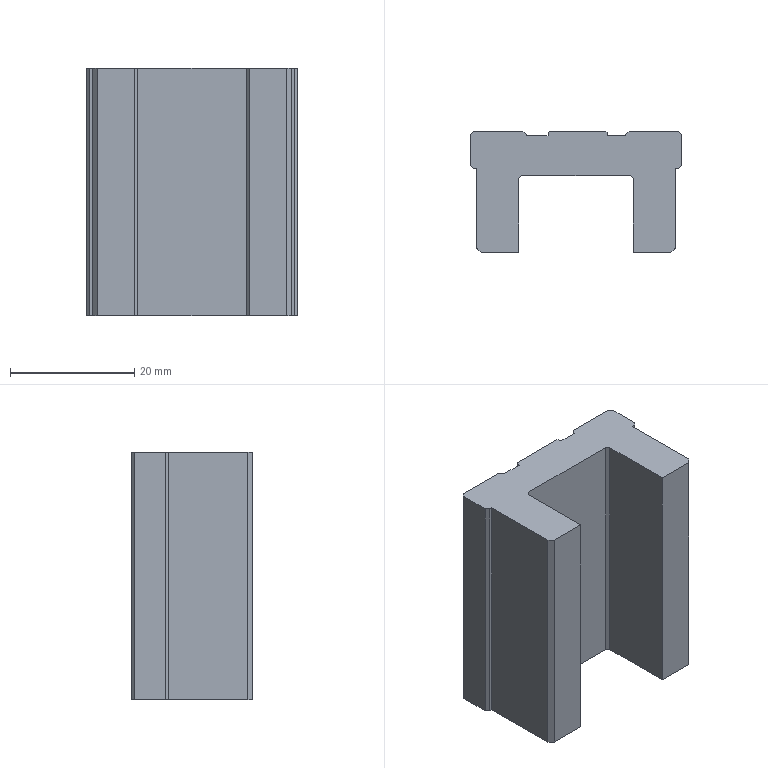Part | STEP file | 8 | 1 solid | 46 faces | box 34 x 19.5 x 39.8 mm | volume 15652 mm3 | plane 38 | cylinder 8 | commonest cylinder face diameters 4 x8
STEP:
#1=CARTESIAN_POINT('',(-13.,24.,-141.));
#2=VERTEX_POINT('',#1);
#3=CARTESIAN_POINT('',(-13.,24.,-145.));
#4=VERTEX_POINT('',#3);
#5=CARTESIAN_POINT('',(-13.,24.,-143.));
#6=DIRECTION('',(0.,-1.,0.));
#7=DIRECTION('',(0.,0.,-1.));
#8=AXIS2_PLACEMENT_3D('',#5,#6,#7);
#9=CIRCLE('',#8,2.);
#10=EDGE_CURVE('',#2,#4,#9,.T.);
#11=ORIENTED_EDGE('',*,*,#10,.F.);
#12=CARTESIAN_POINT('',(-13.,18.,-141.));
#13=VERTEX_POINT('',#12);
#14=CARTESIAN_POINT('',(-13.,24.,-141.));
#15=DIRECTION('',(0.,-1.,0.));
#16=VECTOR('',#15,1000.);
#17=LINE('',#14,#16);
#18=EDGE_CURVE('',#2,#13,#17,.T.);
#19=ORIENTED_EDGE('',*,*,#18,.T.);
#20=CARTESIAN_POINT('',(-13.,18.,-145.));
#21=VERTEX_POINT('',#20);
#22=CARTESIAN_POINT('',(-13.,18.,-143.));
#23=DIRECTION('',(0.,1.,0.));
#24=DIRECTION('',(0.,0.,-1.));
#25=AXIS2_PLACEMENT_3D('',#22,#23,#24);
#26=CIRCLE('',#25,2.);
#27=EDGE_CURVE('',#21,#13,#26,.T.);
#28=ORIENTED_EDGE('',*,*,#27,.F.);
#29=CARTESIAN_POINT('',(-13.,24.,-145.));
#30=DIRECTION('',(0.,-1.,0.));
#31=VECTOR('',#30,1000.);
#32=LINE('',#29,#31);
#33=EDGE_CURVE('',#4,#21,#32,.T.);
#34=ORIENTED_EDGE('',*,*,#33,.F.);
#35=EDGE_LOOP('',(#11,#19,#28,#34));
#36=FACE_OUTER_BOUND('',#35,.T.);
#37=CARTESIAN_POINT('',(-13.,24.,-143.));
#38=DIRECTION('',(0.,-1.,0.));
#39=DIRECTION('',(0.,0.,-1.));
#40=AXIS2_PLACEMENT_3D('',#37,#38,#39);
#41=CYLINDRICAL_SURFACE('',#40,2.);
#42=ADVANCED_FACE('',(#36),#41,.F.);
#43=CARTESIAN_POINT('',(-13.,24.,-115.));
#44=VERTEX_POINT('',#43);
#45=CARTESIAN_POINT('',(-13.,24.,-119.));
#46=VERTEX_POINT('',#45);
#47=CARTESIAN_POINT('',(-13.,24.,-117.));
#48=DIRECTION('',(0.,-1.,0.));
#49=DIRECTION('',(0.,0.,-1.));
#50=AXIS2_PLACEMENT_3D('',#47,#48,#49);
#51=CIRCLE('',#50,2.);
#52=EDGE_CURVE('',#44,#46,#51,.T.);
#53=ORIENTED_EDGE('',*,*,#52,.F.);
#54=CARTESIAN_POINT('',(-13.,18.,-115.));
#55=VERTEX_POINT('',#54);
#56=CARTESIAN_POINT('',(-13.,24.,-115.));
#57=DIRECTION('',(0.,-1.,0.));
#58=VECTOR('',#57,1000.);
#59=LINE('',#56,#58);
#60=EDGE_CURVE('',#44,#55,#59,.T.);
#61=ORIENTED_EDGE('',*,*,#60,.T.);
#62=CARTESIAN_POINT('',(-13.,18.,-119.));
#63=VERTEX_POINT('',#62);
#64=CARTESIAN_POINT('',(-13.,18.,-117.));
#65=DIRECTION('',(0.,1.,0.));
#66=DIRECTION('',(0.,0.,-1.));
#67=AXIS2_PLACEMENT_3D('',#64,#65,#66);
#68=CIRCLE('',#67,2.);
#69=EDGE_CURVE('',#63,#55,#68,.T.);
#70=ORIENTED_EDGE('',*,*,#69,.F.);
#71=CARTESIAN_POINT('',(-13.,24.,-119.));
#72=DIRECTION('',(0.,-1.,0.));
#73=VECTOR('',#72,1000.);
#74=LINE('',#71,#73);
#75=EDGE_CURVE('',#46,#63,#74,.T.);
#76=ORIENTED_EDGE('',*,*,#75,.F.);
#77=EDGE_LOOP('',(#53,#61,#70,#76));
#78=FACE_OUTER_BOUND('',#77,.T.);
#79=CARTESIAN_POINT('',(-13.,24.,-117.));
#80=DIRECTION('',(0.,-1.,0.));
#81=DIRECTION('',(0.,0.,-1.));
#82=AXIS2_PLACEMENT_3D('',#79,#80,#81);
#83=CYLINDRICAL_SURFACE('',#82,2.);
#84=ADVANCED_FACE('',(#78),#83,.F.);
#85=CARTESIAN_POINT('',(13.,24.,-115.));
#86=VERTEX_POINT('',#85);
#87=CARTESIAN_POINT('',(13.,24.,-119.));
#88=VERTEX_POINT('',#87);
#89=CARTESIAN_POINT('',(13.,24.,-117.));
#90=DIRECTION('',(0.,-1.,0.));
#91=DIRECTION('',(0.,0.,-1.));
#92=AXIS2_PLACEMENT_3D('',#89,#90,#91);
#93=CIRCLE('',#92,2.);
#94=EDGE_CURVE('',#86,#88,#93,.T.);
#95=ORIENTED_EDGE('',*,*,#94,.F.);
#96=CARTESIAN_POINT('',(13.,18.,-115.));
#97=VERTEX_POINT('',#96);
#98=CARTESIAN_POINT('',(13.,24.,-115.));
#99=DIRECTION('',(0.,-1.,0.));
#100=VECTOR('',#99,1000.);
#101=LINE('',#98,#100);
#102=EDGE_CURVE('',#86,#97,#101,.T.);
#103=ORIENTED_EDGE('',*,*,#102,.T.);
#104=CARTESIAN_POINT('',(13.,18.,-119.));
#105=VERTEX_POINT('',#104);
#106=CARTESIAN_POINT('',(13.,18.,-117.));
#107=DIRECTION('',(0.,1.,0.));
#108=DIRECTION('',(0.,0.,-1.));
#109=AXIS2_PLACEMENT_3D('',#106,#107,#108);
#110=CIRCLE('',#109,2.);
#111=EDGE_CURVE('',#105,#97,#110,.T.);
#112=ORIENTED_EDGE('',*,*,#111,.F.);
#113=CARTESIAN_POINT('',(13.,24.,-119.));
#114=DIRECTION('',(0.,-1.,0.));
#115=VECTOR('',#114,1000.);
#116=LINE('',#113,#115);
#117=EDGE_CURVE('',#88,#105,#116,.T.);
#118=ORIENTED_EDGE('',*,*,#117,.F.);
#119=EDGE_LOOP('',(#95,#103,#112,#118));
#120=FACE_OUTER_BOUND('',#119,.T.);
#121=CARTESIAN_POINT('',(13.,24.,-117.));
#122=DIRECTION('',(0.,-1.,0.));
#123=DIRECTION('',(0.,0.,-1.));
#124=AXIS2_PLACEMENT_3D('',#121,#122,#123);
#125=CYLINDRICAL_SURFACE('',#124,2.);
#126=ADVANCED_FACE('',(#120),#125,.F.);
#127=CARTESIAN_POINT('',(13.,24.,-141.));
#128=VERTEX_POINT('',#127);
#129=CARTESIAN_POINT('',(13.,24.,-145.));
#130=VERTEX_POINT('',#129);
#131=CARTESIAN_POINT('',(13.,24.,-143.));
#132=DIRECTION('',(0.,-1.,0.));
#133=DIRECTION('',(0.,0.,-1.));
#134=AXIS2_PLACEMENT_3D('',#131,#132,#133);
#135=CIRCLE('',#134,2.);
#136=EDGE_CURVE('',#128,#130,#135,.T.);
#137=ORIENTED_EDGE('',*,*,#136,.F.);
#138=CARTESIAN_POINT('',(13.,18.,-141.));
#139=VERTEX_POINT('',#138);
#140=CARTESIAN_POINT('',(13.,24.,-141.));
#141=DIRECTION('',(0.,-1.,0.));
#142=VECTOR('',#141,1000.);
#143=LINE('',#140,#142);
#144=EDGE_CURVE('',#128,#139,#143,.T.);
#145=ORIENTED_EDGE('',*,*,#144,.T.);
#146=CARTESIAN_POINT('',(13.,18.,-145.));
#147=VERTEX_POINT('',#146);
#148=CARTESIAN_POINT('',(13.,18.,-143.));
#149=DIRECTION('',(0.,1.,0.));
#150=DIRECTION('',(0.,0.,-1.));
#151=AXIS2_PLACEMENT_3D('',#148,#149,#150);
#152=CIRCLE('',#151,2.);
#153=EDGE_CURVE('',#147,#139,#152,.T.);
#154=ORIENTED_EDGE('',*,*,#153,.F.);
#155=CARTESIAN_POINT('',(13.,24.,-145.));
#156=DIRECTION('',(0.,-1.,0.));
#157=VECTOR('',#156,1000.);
#158=LINE('',#155,#157);
#159=EDGE_CURVE('',#130,#147,#158,.T.);
#160=ORIENTED_EDGE('',*,*,#159,.F.);
#161=EDGE_LOOP('',(#137,#145,#154,#160));
#162=FACE_OUTER_BOUND('',#161,.T.);
#163=CARTESIAN_POINT('',(13.,24.,-143.));
#164=DIRECTION('',(0.,-1.,0.));
#165=DIRECTION('',(0.,0.,-1.));
#166=AXIS2_PLACEMENT_3D('',#163,#164,#165);
#167=CYLINDRICAL_SURFACE('',#166,2.);
#168=ADVANCED_FACE('',(#162),#167,.F.);
#169=CARTESIAN_POINT('',(-8.75,16.9,-149.9));
#170=VERTEX_POINT('',#169);
#171=CARTESIAN_POINT('',(8.75,16.9,-149.9));
#172=VERTEX_POINT('',#171);
#173=CARTESIAN_POINT('',(0.,16.9,-149.9));
#174=DIRECTION('',(1.,0.,0.));
#175=VECTOR('',#174,1000.);
#176=LINE('',#173,#175);
#177=EDGE_CURVE('',#170,#172,#176,.T.);
#178=ORIENTED_EDGE('',*,*,#177,.T.);
#179=CARTESIAN_POINT('',(8.75,16.9,-110.1));
#180=VERTEX_POINT('',#179);
#181=CARTESIAN_POINT('',(8.75,16.9,-130.));
#182=DIRECTION('',(0.,0.,1.));
#183=VECTOR('',#182,1000.);
#184=LINE('',#181,#183);
#185=EDGE_CURVE('',#172,#180,#184,.T.);
#186=ORIENTED_EDGE('',*,*,#185,.T.);
#187=CARTESIAN_POINT('',(-8.75,16.9,-110.1));
#188=VERTEX_POINT('',#187);
#189=CARTESIAN_POINT('',(0.,16.9,-110.1));
#190=DIRECTION('',(-1.,0.,0.));
#191=VECTOR('',#190,1000.);
#192=LINE('',#189,#191);
#193=EDGE_CURVE('',#180,#188,#192,.T.);
#194=ORIENTED_EDGE('',*,*,#193,.T.);
#195=CARTESIAN_POINT('',(-8.75,16.9,-130.));
#196=DIRECTION('',(0.,0.,-1.));
#197=VECTOR('',#196,1000.);
#198=LINE('',#195,#197);
#199=EDGE_CURVE('',#188,#170,#198,.T.);
#200=ORIENTED_EDGE('',*,*,#199,.T.);
#201=EDGE_LOOP('',(#178,#186,#194,#200));
#202=FACE_OUTER_BOUND('',#201,.T.);
#203=CARTESIAN_POINT('',(0.,16.9,-130.));
#204=DIRECTION('',(0.,-1.,0.));
#205=DIRECTION('',(0.,0.,-1.));
#206=AXIS2_PLACEMENT_3D('',#203,#204,#205);
#207=PLANE('',#206);
#208=ADVANCED_FACE('',(#202),#207,.T.);
#209=CARTESIAN_POINT('',(9.25,16.4,-149.9));
#210=VERTEX_POINT('',#209);
#211=CARTESIAN_POINT('',(9.,16.65,-149.9));
#212=DIRECTION('',(0.7071,-0.7071,0.));
#213=VECTOR('',#212,1000.);
#214=LINE('',#211,#213);
#215=EDGE_CURVE('',#172,#210,#214,.T.);
#216=ORIENTED_EDGE('',*,*,#215,.T.);
#217=CARTESIAN_POINT('',(9.25,16.4,-110.1));
#218=VERTEX_POINT('',#217);
#219=CARTESIAN_POINT('',(9.25,16.4,-130.));
#220=DIRECTION('',(0.,0.,1.));
#221=VECTOR('',#220,1000.);
#222=LINE('',#219,#221);
#223=EDGE_CURVE('',#210,#218,#222,.T.);
#224=ORIENTED_EDGE('',*,*,#223,.T.);
#225=CARTESIAN_POINT('',(9.,16.65,-110.1));
#226=DIRECTION('',(-0.7071,0.7071,0.));
#227=VECTOR('',#226,1000.);
#228=LINE('',#225,#227);
#229=EDGE_CURVE('',#218,#180,#228,.T.);
#230=ORIENTED_EDGE('',*,*,#229,.T.);
#231=ORIENTED_EDGE('',*,*,#185,.F.);
#232=EDGE_LOOP('',(#216,#224,#230,#231));
#233=FACE_OUTER_BOUND('',#232,.T.);
#234=CARTESIAN_POINT('',(9.,16.65,-130.));
#235=DIRECTION('',(-0.7071,-0.7071,0.));
#236=DIRECTION('',(0.7071,-0.7071,0.));
#237=AXIS2_PLACEMENT_3D('',#234,#235,#236);
#238=PLANE('',#237);
#239=ADVANCED_FACE('',(#233),#238,.T.);
#240=ORIENTED_EDGE('',*,*,#177,.F.);
#241=CARTESIAN_POINT('',(-9.25,16.4,-149.9));
#242=VERTEX_POINT('',#241);
#243=CARTESIAN_POINT('',(-9.25,16.4,-149.9));
#244=DIRECTION('',(0.7071,0.7071,0.));
#245=VECTOR('',#244,1000.);
#246=LINE('',#243,#245);
#247=EDGE_CURVE('',#242,#170,#246,.T.);
#248=ORIENTED_EDGE('',*,*,#247,.F.);
#249=CARTESIAN_POINT('',(-9.25,4.5,-149.9));
#250=VERTEX_POINT('',#249);
#251=CARTESIAN_POINT('',(-9.25,15.226,-149.9));
#252=DIRECTION('',(0.,1.,0.));
#253=VECTOR('',#252,1000.);
#254=LINE('',#251,#253);
#255=EDGE_CURVE('',#250,#242,#254,.T.);
#256=ORIENTED_EDGE('',*,*,#255,.F.);
#257=CARTESIAN_POINT('',(-15.25,4.5,-149.9));
#258=VERTEX_POINT('',#257);
#259=CARTESIAN_POINT('',(0.002327,4.5,-149.9));
#260=DIRECTION('',(1.,0.,0.));
#261=VECTOR('',#260,1000.);
#262=LINE('',#259,#261);
#263=EDGE_CURVE('',#258,#250,#262,.T.);
#264=ORIENTED_EDGE('',*,*,#263,.F.);
#265=CARTESIAN_POINT('',(-16.,5.25,-149.9));
#266=VERTEX_POINT('',#265);
#267=CARTESIAN_POINT('',(-15.625,4.875,-149.9));
#268=DIRECTION('',(0.7071,-0.7071,0.));
#269=VECTOR('',#268,1000.);
#270=LINE('',#267,#269);
#271=EDGE_CURVE('',#266,#258,#270,.T.);
#272=ORIENTED_EDGE('',*,*,#271,.F.);
#273=CARTESIAN_POINT('',(-16.,18.,-149.9));
#274=VERTEX_POINT('',#273);
#275=CARTESIAN_POINT('',(-16.,15.226,-149.9));
#276=DIRECTION('',(0.,-1.,0.));
#277=VECTOR('',#276,1000.);
#278=LINE('',#275,#277);
#279=EDGE_CURVE('',#274,#266,#278,.T.);
#280=ORIENTED_EDGE('',*,*,#279,.F.);
#281=CARTESIAN_POINT('',(-16.5,18.,-149.9));
#282=VERTEX_POINT('',#281);
#283=CARTESIAN_POINT('',(-16.25,18.,-149.9));
#284=DIRECTION('',(1.,0.,0.));
#285=VECTOR('',#284,1000.);
#286=LINE('',#283,#285);
#287=EDGE_CURVE('',#282,#274,#286,.T.);
#288=ORIENTED_EDGE('',*,*,#287,.F.);
#289=CARTESIAN_POINT('',(-17.,18.5,-149.9));
#290=VERTEX_POINT('',#289);
#291=CARTESIAN_POINT('',(-16.75,18.25,-149.9));
#292=DIRECTION('',(0.7071,-0.7071,0.));
#293=VECTOR('',#292,1000.);
#294=LINE('',#291,#293);
#295=EDGE_CURVE('',#290,#282,#294,.T.);
#296=ORIENTED_EDGE('',*,*,#295,.F.);
#297=CARTESIAN_POINT('',(-17.,23.5,-149.9));
#298=VERTEX_POINT('',#297);
#299=CARTESIAN_POINT('',(-17.,15.226,-149.9));
#300=DIRECTION('',(0.,-1.,0.));
#301=VECTOR('',#300,1000.);
#302=LINE('',#299,#301);
#303=EDGE_CURVE('',#298,#290,#302,.T.);
#304=ORIENTED_EDGE('',*,*,#303,.F.);
#305=CARTESIAN_POINT('',(-16.5,24.,-149.9));
#306=VERTEX_POINT('',#305);
#307=CARTESIAN_POINT('',(-16.75,23.75,-149.9));
#308=DIRECTION('',(-0.7071,-0.7071,0.));
#309=VECTOR('',#308,1000.);
#310=LINE('',#307,#309);
#311=EDGE_CURVE('',#306,#298,#310,.T.);
#312=ORIENTED_EDGE('',*,*,#311,.F.);
#313=CARTESIAN_POINT('',(-8.707,24.,-149.9));
#314=VERTEX_POINT('',#313);
#315=CARTESIAN_POINT('',(0.002327,24.,-149.9));
#316=DIRECTION('',(-1.,0.,0.));
#317=VECTOR('',#316,1000.);
#318=LINE('',#315,#317);
#319=EDGE_CURVE('',#314,#306,#318,.T.);
#320=ORIENTED_EDGE('',*,*,#319,.F.);
#321=CARTESIAN_POINT('',(-8.,23.5,-149.9));
#322=VERTEX_POINT('',#321);
#323=CARTESIAN_POINT('',(-8.354,23.75,-149.9));
#324=DIRECTION('',(-0.8165,0.5774,0.));
#325=VECTOR('',#324,1000.);
#326=LINE('',#323,#325);
#327=EDGE_CURVE('',#322,#314,#326,.T.);
#328=ORIENTED_EDGE('',*,*,#327,.F.);
#329=CARTESIAN_POINT('',(-8.,23.3,-149.9));
#330=VERTEX_POINT('',#329);
#331=CARTESIAN_POINT('',(-8.,23.4,-149.9));
#332=DIRECTION('',(0.,1.,0.));
#333=VECTOR('',#332,1000.);
#334=LINE('',#331,#333);
#335=EDGE_CURVE('',#330,#322,#334,.T.);
#336=ORIENTED_EDGE('',*,*,#335,.F.);
#337=CARTESIAN_POINT('',(-4.5,23.3,-149.9));
#338=VERTEX_POINT('',#337);
#339=CARTESIAN_POINT('',(0.002327,23.3,-149.9));
#340=DIRECTION('',(-1.,0.,0.));
#341=VECTOR('',#340,1000.);
#342=LINE('',#339,#341);
#343=EDGE_CURVE('',#338,#330,#342,.T.);
#344=ORIENTED_EDGE('',*,*,#343,.F.);
#345=CARTESIAN_POINT('',(-4.5,23.8,-149.9));
#346=VERTEX_POINT('',#345);
#347=CARTESIAN_POINT('',(-4.5,23.55,-149.9));
#348=DIRECTION('',(0.,-1.,0.));
#349=VECTOR('',#348,1000.);
#350=LINE('',#347,#349);
#351=EDGE_CURVE('',#346,#338,#350,.T.);
#352=ORIENTED_EDGE('',*,*,#351,.F.);
#353=CARTESIAN_POINT('',(-4.3,24.,-149.9));
#354=VERTEX_POINT('',#353);
#355=CARTESIAN_POINT('',(-4.4,23.9,-149.9));
#356=DIRECTION('',(-0.7071,-0.7071,0.));
#357=VECTOR('',#356,1000.);
#358=LINE('',#355,#357);
#359=EDGE_CURVE('',#354,#346,#358,.T.);
#360=ORIENTED_EDGE('',*,*,#359,.F.);
#361=CARTESIAN_POINT('',(4.8,24.,-149.9));
#362=VERTEX_POINT('',#361);
#363=CARTESIAN_POINT('',(0.002327,24.,-149.9));
#364=DIRECTION('',(-1.,0.,0.));
#365=VECTOR('',#364,1000.);
#366=LINE('',#363,#365);
#367=EDGE_CURVE('',#362,#354,#366,.T.);
#368=ORIENTED_EDGE('',*,*,#367,.F.);
#369=CARTESIAN_POINT('',(5.,23.8,-149.9));
#370=VERTEX_POINT('',#369);
#371=CARTESIAN_POINT('',(4.9,23.9,-149.9));
#372=DIRECTION('',(-0.7071,0.7071,0.));
#373=VECTOR('',#372,1000.);
#374=LINE('',#371,#373);
#375=EDGE_CURVE('',#370,#362,#374,.T.);
#376=ORIENTED_EDGE('',*,*,#375,.F.);
#377=CARTESIAN_POINT('',(5.,23.3,-149.9));
#378=VERTEX_POINT('',#377);
#379=CARTESIAN_POINT('',(5.,23.55,-149.9));
#380=DIRECTION('',(0.,1.,0.));
#381=VECTOR('',#380,1000.);
#382=LINE('',#379,#381);
#383=EDGE_CURVE('',#378,#370,#382,.T.);
#384=ORIENTED_EDGE('',*,*,#383,.F.);
#385=CARTESIAN_POINT('',(8.,23.3,-149.9));
#386=VERTEX_POINT('',#385);
#387=CARTESIAN_POINT('',(0.002327,23.3,-149.9));
#388=DIRECTION('',(-1.,0.,0.));
#389=VECTOR('',#388,1000.);
#390=LINE('',#387,#389);
#391=EDGE_CURVE('',#386,#378,#390,.T.);
#392=ORIENTED_EDGE('',*,*,#391,.F.);
#393=CARTESIAN_POINT('',(8.,23.5,-149.9));
#394=VERTEX_POINT('',#393);
#395=CARTESIAN_POINT('',(8.,23.4,-149.9));
#396=DIRECTION('',(0.,-1.,0.));
#397=VECTOR('',#396,1000.);
#398=LINE('',#395,#397);
#399=EDGE_CURVE('',#394,#386,#398,.T.);
#400=ORIENTED_EDGE('',*,*,#399,.F.);
#401=CARTESIAN_POINT('',(8.707,24.,-149.9));
#402=VERTEX_POINT('',#401);
#403=CARTESIAN_POINT('',(8.354,23.75,-149.9));
#404=DIRECTION('',(-0.8165,-0.5774,0.));
#405=VECTOR('',#404,1000.);
#406=LINE('',#403,#405);
#407=EDGE_CURVE('',#402,#394,#406,.T.);
#408=ORIENTED_EDGE('',*,*,#407,.F.);
#409=CARTESIAN_POINT('',(16.5,24.,-149.9));
#410=VERTEX_POINT('',#409);
#411=CARTESIAN_POINT('',(0.002327,24.,-149.9));
#412=DIRECTION('',(-1.,0.,0.));
#413=VECTOR('',#412,1000.);
#414=LINE('',#411,#413);
#415=EDGE_CURVE('',#410,#402,#414,.T.);
#416=ORIENTED_EDGE('',*,*,#415,.F.);
#417=CARTESIAN_POINT('',(17.,23.5,-149.9));
#418=VERTEX_POINT('',#417);
#419=CARTESIAN_POINT('',(16.75,23.75,-149.9));
#420=DIRECTION('',(-0.7071,0.7071,0.));
#421=VECTOR('',#420,1000.);
#422=LINE('',#419,#421);
#423=EDGE_CURVE('',#418,#410,#422,.T.);
#424=ORIENTED_EDGE('',*,*,#423,.F.);
#425=CARTESIAN_POINT('',(17.,18.5,-149.9));
#426=VERTEX_POINT('',#425);
#427=CARTESIAN_POINT('',(17.,15.226,-149.9));
#428=DIRECTION('',(0.,1.,0.));
#429=VECTOR('',#428,1000.);
#430=LINE('',#427,#429);
#431=EDGE_CURVE('',#426,#418,#430,.T.);
#432=ORIENTED_EDGE('',*,*,#431,.F.);
#433=CARTESIAN_POINT('',(16.5,18.,-149.9));
#434=VERTEX_POINT('',#433);
#435=CARTESIAN_POINT('',(16.75,18.25,-149.9));
#436=DIRECTION('',(0.7071,0.7071,0.));
#437=VECTOR('',#436,1000.);
#438=LINE('',#435,#437);
#439=EDGE_CURVE('',#434,#426,#438,.T.);
#440=ORIENTED_EDGE('',*,*,#439,.F.);
#441=CARTESIAN_POINT('',(16.,18.,-149.9));
#442=VERTEX_POINT('',#441);
#443=CARTESIAN_POINT('',(16.25,18.,-149.9));
#444=DIRECTION('',(1.,0.,0.));
#445=VECTOR('',#444,1000.);
#446=LINE('',#443,#445);
#447=EDGE_CURVE('',#442,#434,#446,.T.);
#448=ORIENTED_EDGE('',*,*,#447,.F.);
#449=CARTESIAN_POINT('',(16.,5.25,-149.9));
#450=VERTEX_POINT('',#449);
#451=CARTESIAN_POINT('',(16.,15.226,-149.9));
#452=DIRECTION('',(0.,1.,0.));
#453=VECTOR('',#452,1000.);
#454=LINE('',#451,#453);
#455=EDGE_CURVE('',#450,#442,#454,.T.);
#456=ORIENTED_EDGE('',*,*,#455,.F.);
#457=CARTESIAN_POINT('',(15.25,4.5,-149.9));
#458=VERTEX_POINT('',#457);
#459=CARTESIAN_POINT('',(15.625,4.875,-149.9));
#460=DIRECTION('',(0.7071,0.7071,0.));
#461=VECTOR('',#460,1000.);
#462=LINE('',#459,#461);
#463=EDGE_CURVE('',#458,#450,#462,.T.);
#464=ORIENTED_EDGE('',*,*,#463,.F.);
#465=CARTESIAN_POINT('',(9.25,4.5,-149.9));
#466=VERTEX_POINT('',#465);
#467=CARTESIAN_POINT('',(0.002327,4.5,-149.9));
#468=DIRECTION('',(1.,0.,0.));
#469=VECTOR('',#468,1000.);
#470=LINE('',#467,#469);
#471=EDGE_CURVE('',#466,#458,#470,.T.);
#472=ORIENTED_EDGE('',*,*,#471,.F.);
#473=CARTESIAN_POINT('',(9.25,15.226,-149.9));
#474=DIRECTION('',(0.,-1.,0.));
#475=VECTOR('',#474,1000.);
#476=LINE('',#473,#475);
#477=EDGE_CURVE('',#210,#466,#476,.T.);
#478=ORIENTED_EDGE('',*,*,#477,.F.);
#479=ORIENTED_EDGE('',*,*,#215,.F.);
#480=EDGE_LOOP('',(#240,#248,#256,#264,#272,#280,#288,#296,#304,#312,#320,#328,#336,#344,#352,#360,#368,#376,#384,#392,#400,#408,#416,#424,#432,#440,#448,#456,#464,#472,#478,#479));
#481=FACE_OUTER_BOUND('',#480,.T.);
#482=CARTESIAN_POINT('',(0.002327,15.226,-149.9));
#483=DIRECTION('',(0.,0.,1.));
#484=DIRECTION('',(0.,-1.,0.));
#485=AXIS2_PLACEMENT_3D('',#482,#483,#484);
#486=PLANE('',#485);
#487=ADVANCED_FACE('',(#481),#486,.F.);
#488=ORIENTED_EDGE('',*,*,#247,.T.);
#489=ORIENTED_EDGE('',*,*,#199,.F.);
#490=CARTESIAN_POINT('',(-9.25,16.4,-110.1));
#491=VERTEX_POINT('',#490);
#492=CARTESIAN_POINT('',(-9.,16.65,-110.1));
#493=DIRECTION('',(-0.7071,-0.7071,0.));
#494=VECTOR('',#493,1000.);
#495=LINE('',#492,#494);
#496=EDGE_CURVE('',#188,#491,#495,.T.);
#497=ORIENTED_EDGE('',*,*,#496,.T.);
#498=CARTESIAN_POINT('',(-9.25,16.4,-130.));
#499=DIRECTION('',(0.,0.,-1.));
#500=VECTOR('',#499,1000.);
#501=LINE('',#498,#500);
#502=EDGE_CURVE('',#491,#242,#501,.T.);
#503=ORIENTED_EDGE('',*,*,#502,.T.);
#504=EDGE_LOOP('',(#488,#489,#497,#503));
#505=FACE_OUTER_BOUND('',#504,.T.);
#506=CARTESIAN_POINT('',(-9.,16.65,-130.));
#507=DIRECTION('',(0.7071,-0.7071,0.));
#508=DIRECTION('',(0.7071,0.7071,0.));
#509=AXIS2_PLACEMENT_3D('',#506,#507,#508);
#510=PLANE('',#509);
#511=ADVANCED_FACE('',(#505),#510,.T.);
#512=CARTESIAN_POINT('',(-15.25,4.5,-110.1));
#513=VERTEX_POINT('',#512);
#514=CARTESIAN_POINT('',(-9.25,4.5,-110.1));
#515=VERTEX_POINT('',#514);
#516=CARTESIAN_POINT('',(0.002327,4.5,-110.1));
#517=DIRECTION('',(1.,0.,0.));
#518=VECTOR('',#517,1000.);
#519=LINE('',#516,#518);
#520=EDGE_CURVE('',#513,#515,#519,.T.);
#521=ORIENTED_EDGE('',*,*,#520,.T.);
#522=CARTESIAN_POINT('',(-9.25,15.226,-110.1));
#523=DIRECTION('',(0.,1.,0.));
#524=VECTOR('',#523,1000.);
#525=LINE('',#522,#524);
#526=EDGE_CURVE('',#515,#491,#525,.T.);
#527=ORIENTED_EDGE('',*,*,#526,.T.);
#528=ORIENTED_EDGE('',*,*,#496,.F.);
#529=ORIENTED_EDGE('',*,*,#193,.F.);
#530=ORIENTED_EDGE('',*,*,#229,.F.);
#531=CARTESIAN_POINT('',(9.25,4.5,-110.1));
#532=VERTEX_POINT('',#531);
#533=CARTESIAN_POINT('',(9.25,15.226,-110.1));
#534=DIRECTION('',(0.,-1.,0.));
#535=VECTOR('',#534,1000.);
#536=LINE('',#533,#535);
#537=EDGE_CURVE('',#218,#532,#536,.T.);
#538=ORIENTED_EDGE('',*,*,#537,.T.);
#539=CARTESIAN_POINT('',(15.25,4.5,-110.1));
#540=VERTEX_POINT('',#539);
#541=CARTESIAN_POINT('',(0.002327,4.5,-110.1));
#542=DIRECTION('',(1.,0.,0.));
#543=VECTOR('',#542,1000.);
#544=LINE('',#541,#543);
#545=EDGE_CURVE('',#532,#540,#544,.T.);
#546=ORIENTED_EDGE('',*,*,#545,.T.);
#547=CARTESIAN_POINT('',(16.,5.25,-110.1));
#548=VERTEX_POINT('',#547);
#549=CARTESIAN_POINT('',(15.625,4.875,-110.1));
#550=DIRECTION('',(-0.7071,-0.7071,0.));
#551=VECTOR('',#550,1000.);
#552=LINE('',#549,#551);
#553=EDGE_CURVE('',#548,#540,#552,.T.);
#554=ORIENTED_EDGE('',*,*,#553,.F.);
#555=CARTESIAN_POINT('',(16.,18.,-110.1));
#556=VERTEX_POINT('',#555);
#557=CARTESIAN_POINT('',(16.,15.226,-110.1));
#558=DIRECTION('',(0.,1.,0.));
#559=VECTOR('',#558,1000.);
#560=LINE('',#557,#559);
#561=EDGE_CURVE('',#548,#556,#560,.T.);
#562=ORIENTED_EDGE('',*,*,#561,.T.);
#563=CARTESIAN_POINT('',(16.5,18.,-110.1));
#564=VERTEX_POINT('',#563);
#565=CARTESIAN_POINT('',(16.25,18.,-110.1));
#566=DIRECTION('',(-1.,0.,0.));
#567=VECTOR('',#566,1000.);
#568=LINE('',#565,#567);
#569=EDGE_CURVE('',#564,#556,#568,.T.);
#570=ORIENTED_EDGE('',*,*,#569,.F.);
#571=CARTESIAN_POINT('',(17.,18.5,-110.1));
#572=VERTEX_POINT('',#571);
#573=CARTESIAN_POINT('',(16.75,18.25,-110.1));
#574=DIRECTION('',(-0.7071,-0.7071,0.));
#575=VECTOR('',#574,1000.);
#576=LINE('',#573,#575);
#577=EDGE_CURVE('',#572,#564,#576,.T.);
#578=ORIENTED_EDGE('',*,*,#577,.F.);
#579=CARTESIAN_POINT('',(17.,23.5,-110.1));
#580=VERTEX_POINT('',#579);
#581=CARTESIAN_POINT('',(17.,15.226,-110.1));
#582=DIRECTION('',(0.,1.,0.));
#583=VECTOR('',#582,1000.);
#584=LINE('',#581,#583);
#585=EDGE_CURVE('',#572,#580,#584,.T.);
#586=ORIENTED_EDGE('',*,*,#585,.T.);
#587=CARTESIAN_POINT('',(16.5,24.,-110.1));
#588=VERTEX_POINT('',#587);
#589=CARTESIAN_POINT('',(16.75,23.75,-110.1));
#590=DIRECTION('',(0.7071,-0.7071,0.));
#591=VECTOR('',#590,1000.);
#592=LINE('',#589,#591);
#593=EDGE_CURVE('',#588,#580,#592,.T.);
#594=ORIENTED_EDGE('',*,*,#593,.F.);
#595=CARTESIAN_POINT('',(8.707,24.,-110.1));
#596=VERTEX_POINT('',#595);
#597=CARTESIAN_POINT('',(0.002327,24.,-110.1));
#598=DIRECTION('',(-1.,0.,0.));
#599=VECTOR('',#598,1000.);
#600=LINE('',#597,#599);
#601=EDGE_CURVE('',#588,#596,#600,.T.);
#602=ORIENTED_EDGE('',*,*,#601,.T.);
#603=CARTESIAN_POINT('',(8.,23.5,-110.1));
#604=VERTEX_POINT('',#603);
#605=CARTESIAN_POINT('',(8.354,23.75,-110.1));
#606=DIRECTION('',(0.8165,0.5774,0.));
#607=VECTOR('',#606,1000.);
#608=LINE('',#605,#607);
#609=EDGE_CURVE('',#604,#596,#608,.T.);
#610=ORIENTED_EDGE('',*,*,#609,.F.);
#611=CARTESIAN_POINT('',(8.,23.3,-110.1));
#612=VERTEX_POINT('',#611);
#613=CARTESIAN_POINT('',(8.,23.4,-110.1));
#614=DIRECTION('',(0.,1.,0.));
#615=VECTOR('',#614,1000.);
#616=LINE('',#613,#615);
#617=EDGE_CURVE('',#612,#604,#616,.T.);
#618=ORIENTED_EDGE('',*,*,#617,.F.);
#619=CARTESIAN_POINT('',(5.,23.3,-110.1));
#620=VERTEX_POINT('',#619);
#621=CARTESIAN_POINT('',(0.002327,23.3,-110.1));
#622=DIRECTION('',(-1.,0.,0.));
#623=VECTOR('',#622,1000.);
#624=LINE('',#621,#623);
#625=EDGE_CURVE('',#612,#620,#624,.T.);
#626=ORIENTED_EDGE('',*,*,#625,.T.);
#627=CARTESIAN_POINT('',(5.,23.8,-110.1));
#628=VERTEX_POINT('',#627);
#629=CARTESIAN_POINT('',(5.,23.55,-110.1));
#630=DIRECTION('',(0.,-1.,0.));
#631=VECTOR('',#630,1000.);
#632=LINE('',#629,#631);
#633=EDGE_CURVE('',#628,#620,#632,.T.);
#634=ORIENTED_EDGE('',*,*,#633,.F.);
#635=CARTESIAN_POINT('',(4.8,24.,-110.1));
#636=VERTEX_POINT('',#635);
#637=CARTESIAN_POINT('',(4.9,23.9,-110.1));
#638=DIRECTION('',(0.7071,-0.7071,0.));
#639=VECTOR('',#638,1000.);
#640=LINE('',#637,#639);
#641=EDGE_CURVE('',#636,#628,#640,.T.);
#642=ORIENTED_EDGE('',*,*,#641,.F.);
#643=CARTESIAN_POINT('',(-4.3,24.,-110.1));
#644=VERTEX_POINT('',#643);
#645=CARTESIAN_POINT('',(0.002327,24.,-110.1));
#646=DIRECTION('',(-1.,0.,0.));
#647=VECTOR('',#646,1000.);
#648=LINE('',#645,#647);
#649=EDGE_CURVE('',#636,#644,#648,.T.);
#650=ORIENTED_EDGE('',*,*,#649,.T.);
#651=CARTESIAN_POINT('',(-4.5,23.8,-110.1));
#652=VERTEX_POINT('',#651);
#653=CARTESIAN_POINT('',(-4.4,23.9,-110.1));
#654=DIRECTION('',(0.7071,0.7071,0.));
#655=VECTOR('',#654,1000.);
#656=LINE('',#653,#655);
#657=EDGE_CURVE('',#652,#644,#656,.T.);
#658=ORIENTED_EDGE('',*,*,#657,.F.);
#659=CARTESIAN_POINT('',(-4.5,23.3,-110.1));
#660=VERTEX_POINT('',#659);
#661=CARTESIAN_POINT('',(-4.5,23.55,-110.1));
#662=DIRECTION('',(0.,1.,0.));
#663=VECTOR('',#662,1000.);
#664=LINE('',#661,#663);
#665=EDGE_CURVE('',#660,#652,#664,.T.);
#666=ORIENTED_EDGE('',*,*,#665,.F.);
#667=CARTESIAN_POINT('',(-8.,23.3,-110.1));
#668=VERTEX_POINT('',#667);
#669=CARTESIAN_POINT('',(0.002327,23.3,-110.1));
#670=DIRECTION('',(-1.,0.,0.));
#671=VECTOR('',#670,1000.);
#672=LINE('',#669,#671);
#673=EDGE_CURVE('',#660,#668,#672,.T.);
#674=ORIENTED_EDGE('',*,*,#673,.T.);
#675=CARTESIAN_POINT('',(-8.,23.5,-110.1));
#676=VERTEX_POINT('',#675);
#677=CARTESIAN_POINT('',(-8.,23.4,-110.1));
#678=DIRECTION('',(0.,-1.,0.));
#679=VECTOR('',#678,1000.);
#680=LINE('',#677,#679);
#681=EDGE_CURVE('',#676,#668,#680,.T.);
#682=ORIENTED_EDGE('',*,*,#681,.F.);
#683=CARTESIAN_POINT('',(-8.707,24.,-110.1));
#684=VERTEX_POINT('',#683);
#685=CARTESIAN_POINT('',(-8.354,23.75,-110.1));
#686=DIRECTION('',(0.8165,-0.5774,0.));
#687=VECTOR('',#686,1000.);
#688=LINE('',#685,#687);
#689=EDGE_CURVE('',#684,#676,#688,.T.);
#690=ORIENTED_EDGE('',*,*,#689,.F.);
#691=CARTESIAN_POINT('',(-16.5,24.,-110.1));
#692=VERTEX_POINT('',#691);
#693=CARTESIAN_POINT('',(0.002327,24.,-110.1));
#694=DIRECTION('',(-1.,0.,0.));
#695=VECTOR('',#694,1000.);
#696=LINE('',#693,#695);
#697=EDGE_CURVE('',#684,#692,#696,.T.);
#698=ORIENTED_EDGE('',*,*,#697,.T.);
#699=CARTESIAN_POINT('',(-17.,23.5,-110.1));
#700=VERTEX_POINT('',#699);
#701=CARTESIAN_POINT('',(-16.75,23.75,-110.1));
#702=DIRECTION('',(0.7071,0.7071,0.));
#703=VECTOR('',#702,1000.);
#704=LINE('',#701,#703);
#705=EDGE_CURVE('',#700,#692,#704,.T.);
#706=ORIENTED_EDGE('',*,*,#705,.F.);
#707=CARTESIAN_POINT('',(-17.,18.5,-110.1));
#708=VERTEX_POINT('',#707);
#709=CARTESIAN_POINT('',(-17.,15.226,-110.1));
#710=DIRECTION('',(0.,-1.,0.));
#711=VECTOR('',#710,1000.);
#712=LINE('',#709,#711);
#713=EDGE_CURVE('',#700,#708,#712,.T.);
#714=ORIENTED_EDGE('',*,*,#713,.T.);
#715=CARTESIAN_POINT('',(-16.5,18.,-110.1));
#716=VERTEX_POINT('',#715);
#717=CARTESIAN_POINT('',(-16.75,18.25,-110.1));
#718=DIRECTION('',(-0.7071,0.7071,0.));
#719=VECTOR('',#718,1000.);
#720=LINE('',#717,#719);
#721=EDGE_CURVE('',#716,#708,#720,.T.);
#722=ORIENTED_EDGE('',*,*,#721,.F.);
#723=CARTESIAN_POINT('',(-16.,18.,-110.1));
#724=VERTEX_POINT('',#723);
#725=CARTESIAN_POINT('',(-16.25,18.,-110.1));
#726=DIRECTION('',(-1.,0.,0.));
#727=VECTOR('',#726,1000.);
#728=LINE('',#725,#727);
#729=EDGE_CURVE('',#724,#716,#728,.T.);
#730=ORIENTED_EDGE('',*,*,#729,.F.);
#731=CARTESIAN_POINT('',(-16.,5.25,-110.1));
#732=VERTEX_POINT('',#731);
#733=CARTESIAN_POINT('',(-16.,15.226,-110.1));
#734=DIRECTION('',(0.,-1.,0.));
#735=VECTOR('',#734,1000.);
#736=LINE('',#733,#735);
#737=EDGE_CURVE('',#724,#732,#736,.T.);
#738=ORIENTED_EDGE('',*,*,#737,.T.);
#739=CARTESIAN_POINT('',(-15.625,4.875,-110.1));
#740=DIRECTION('',(-0.7071,0.7071,0.));
#741=VECTOR('',#740,1000.);
#742=LINE('',#739,#741);
#743=EDGE_CURVE('',#513,#732,#742,.T.);
#744=ORIENTED_EDGE('',*,*,#743,.F.);
#745=EDGE_LOOP('',(#521,#527,#528,#529,#530,#538,#546,#554,#562,#570,#578,#586,#594,#602,#610,#618,#626,#634,#642,#650,#658,#666,#674,#682,#690,#698,#706,#714,#722,#730,#738,#744));
#746=FACE_OUTER_BOUND('',#745,.T.);
#747=CARTESIAN_POINT('',(0.002327,15.226,-110.1));
#748=DIRECTION('',(0.,0.,1.));
#749=DIRECTION('',(0.,-1.,0.));
#750=AXIS2_PLACEMENT_3D('',#747,#748,#749);
#751=PLANE('',#750);
#752=ADVANCED_FACE('',(#746),#751,.T.);
#753=ORIENTED_EDGE('',*,*,#477,.T.);
#754=CARTESIAN_POINT('',(9.25,4.5,-130.));
#755=DIRECTION('',(0.,0.,1.));
#756=VECTOR('',#755,1000.);
#757=LINE('',#754,#756);
#758=EDGE_CURVE('',#466,#532,#757,.T.);
#759=ORIENTED_EDGE('',*,*,#758,.T.);
#760=ORIENTED_EDGE('',*,*,#537,.F.);
#761=ORIENTED_EDGE('',*,*,#223,.F.);
#762=EDGE_LOOP('',(#753,#759,#760,#761));
#763=FACE_OUTER_BOUND('',#762,.T.);
#764=CARTESIAN_POINT('',(9.25,10.45,-130.));
#765=DIRECTION('',(-1.,0.,0.));
#766=DIRECTION('',(0.,0.,1.));
#767=AXIS2_PLACEMENT_3D('',#764,#765,#766);
#768=PLANE('',#767);
#769=ADVANCED_FACE('',(#763),#768,.T.);
#770=ORIENTED_EDGE('',*,*,#255,.T.);
#771=ORIENTED_EDGE('',*,*,#502,.F.);
#772=ORIENTED_EDGE('',*,*,#526,.F.);
#773=CARTESIAN_POINT('',(-9.25,4.5,-130.));
#774=DIRECTION('',(0.,0.,-1.));
#775=VECTOR('',#774,1000.);
#776=LINE('',#773,#775);
#777=EDGE_CURVE('',#515,#250,#776,.T.);
#778=ORIENTED_EDGE('',*,*,#777,.T.);
#779=EDGE_LOOP('',(#770,#771,#772,#778));
#780=FACE_OUTER_BOUND('',#779,.T.);
#781=CARTESIAN_POINT('',(-9.25,10.45,-130.));
#782=DIRECTION('',(1.,0.,0.));
#783=DIRECTION('',(0.,0.,-1.));
#784=AXIS2_PLACEMENT_3D('',#781,#782,#783);
#785=PLANE('',#784);
#786=ADVANCED_FACE('',(#780),#785,.T.);
#787=ORIENTED_EDGE('',*,*,#263,.T.);
#788=ORIENTED_EDGE('',*,*,#777,.F.);
#789=ORIENTED_EDGE('',*,*,#520,.F.);
#790=CARTESIAN_POINT('',(-15.25,4.5,-130.));
#791=DIRECTION('',(0.,0.,-1.));
#792=VECTOR('',#791,1000.);
#793=LINE('',#790,#792);
#794=EDGE_CURVE('',#513,#258,#793,.T.);
#795=ORIENTED_EDGE('',*,*,#794,.T.);
#796=EDGE_LOOP('',(#787,#788,#789,#795));
#797=FACE_OUTER_BOUND('',#796,.T.);
#798=CARTESIAN_POINT('',(-12.25,4.5,-130.));
#799=DIRECTION('',(0.,-1.,0.));
#800=DIRECTION('',(0.,0.,-1.));
#801=AXIS2_PLACEMENT_3D('',#798,#799,#800);
#802=PLANE('',#801);
#803=ADVANCED_FACE('',(#797),#802,.T.);
#804=CARTESIAN_POINT('',(-16.,5.25,-130.));
#805=DIRECTION('',(0.,0.,1.));
#806=VECTOR('',#805,1000.);
#807=LINE('',#804,#806);
#808=EDGE_CURVE('',#266,#732,#807,.T.);
#809=ORIENTED_EDGE('',*,*,#808,.T.);
#810=ORIENTED_EDGE('',*,*,#737,.F.);
#811=CARTESIAN_POINT('',(-16.,18.,-130.));
#812=DIRECTION('',(0.,0.,-1.));
#813=VECTOR('',#812,1000.);
#814=LINE('',#811,#813);
#815=EDGE_CURVE('',#724,#274,#814,.T.);
#816=ORIENTED_EDGE('',*,*,#815,.T.);
#817=ORIENTED_EDGE('',*,*,#279,.T.);
#818=EDGE_LOOP('',(#809,#810,#816,#817));
#819=FACE_OUTER_BOUND('',#818,.T.);
#820=CARTESIAN_POINT('',(-16.,13.9,-130.));
#821=DIRECTION('',(-1.,0.,0.));
#822=DIRECTION('',(0.,0.,1.));
#823=AXIS2_PLACEMENT_3D('',#820,#821,#822);
#824=PLANE('',#823);
#825=ADVANCED_FACE('',(#819),#824,.T.);
#826=ORIENTED_EDGE('',*,*,#303,.T.);
#827=CARTESIAN_POINT('',(-17.,18.5,-130.));
#828=DIRECTION('',(0.,0.,1.));
#829=VECTOR('',#828,1000.);
#830=LINE('',#827,#829);
#831=EDGE_CURVE('',#290,#708,#830,.T.);
#832=ORIENTED_EDGE('',*,*,#831,.T.);
#833=ORIENTED_EDGE('',*,*,#713,.F.);
#834=CARTESIAN_POINT('',(-17.,23.5,-130.));
#835=DIRECTION('',(0.,0.,-1.));
#836=VECTOR('',#835,1000.);
#837=LINE('',#834,#836);
#838=EDGE_CURVE('',#700,#298,#837,.T.);
#839=ORIENTED_EDGE('',*,*,#838,.T.);
#840=EDGE_LOOP('',(#826,#832,#833,#839));
#841=FACE_OUTER_BOUND('',#840,.T.);
#842=CARTESIAN_POINT('',(-17.,21.,-130.));
#843=DIRECTION('',(-1.,0.,0.));
#844=DIRECTION('',(0.,0.,1.));
#845=AXIS2_PLACEMENT_3D('',#842,#843,#844);
#846=PLANE('',#845);
#847=ADVANCED_FACE('',(#841),#846,.T.);
#848=CARTESIAN_POINT('',(-13.,24.,-143.));
#849=DIRECTION('',(0.,-1.,0.));
#850=DIRECTION('',(0.,0.,-1.));
#851=AXIS2_PLACEMENT_3D('',#848,#849,#850);
#852=CIRCLE('',#851,2.);
#853=EDGE_CURVE('',#4,#2,#852,.T.);
#854=ORIENTED_EDGE('',*,*,#853,.T.);
#855=ORIENTED_EDGE('',*,*,#10,.T.);
#856=EDGE_LOOP('',(#854,#855));
#857=FACE_BOUND('',#856,.T.);
#858=CARTESIAN_POINT('',(-13.,24.,-117.));
#859=DIRECTION('',(0.,-1.,0.));
#860=DIRECTION('',(0.,0.,-1.));
#861=AXIS2_PLACEMENT_3D('',#858,#859,#860);
#862=CIRCLE('',#861,2.);
#863=EDGE_CURVE('',#46,#44,#862,.T.);
#864=ORIENTED_EDGE('',*,*,#863,.T.);
#865=ORIENTED_EDGE('',*,*,#52,.T.);
#866=EDGE_LOOP('',(#864,#865));
#867=FACE_BOUND('',#866,.T.);
#868=ORIENTED_EDGE('',*,*,#319,.T.);
#869=CARTESIAN_POINT('',(-16.5,24.,-130.));
#870=DIRECTION('',(0.,0.,1.));
#871=VECTOR('',#870,1000.);
#872=LINE('',#869,#871);
#873=EDGE_CURVE('',#306,#692,#872,.T.);
#874=ORIENTED_EDGE('',*,*,#873,.T.);
#875=ORIENTED_EDGE('',*,*,#697,.F.);
#876=CARTESIAN_POINT('',(-8.707,24.,-130.));
#877=DIRECTION('',(0.,0.,-1.));
#878=VECTOR('',#877,1000.);
#879=LINE('',#876,#878);
#880=EDGE_CURVE('',#684,#314,#879,.T.);
#881=ORIENTED_EDGE('',*,*,#880,.T.);
#882=EDGE_LOOP('',(#868,#874,#875,#881));
#883=FACE_OUTER_BOUND('',#882,.T.);
#884=CARTESIAN_POINT('',(-12.604,24.,-130.));
#885=DIRECTION('',(0.,1.,0.));
#886=DIRECTION('',(0.,0.,1.));
#887=AXIS2_PLACEMENT_3D('',#884,#885,#886);
#888=PLANE('',#887);
#889=ADVANCED_FACE('',(#857,#867,#883),#888,.T.);
#890=CARTESIAN_POINT('',(-4.5,23.3,-130.));
#891=DIRECTION('',(0.,0.,-1.));
#892=VECTOR('',#891,1000.);
#893=LINE('',#890,#892);
#894=EDGE_CURVE('',#660,#338,#893,.T.);
#895=ORIENTED_EDGE('',*,*,#894,.T.);
#896=ORIENTED_EDGE('',*,*,#343,.T.);
#897=CARTESIAN_POINT('',(-8.,23.3,-130.));
#898=DIRECTION('',(0.,0.,1.));
#899=VECTOR('',#898,1000.);
#900=LINE('',#897,#899);
#901=EDGE_CURVE('',#330,#668,#900,.T.);
#902=ORIENTED_EDGE('',*,*,#901,.T.);
#903=ORIENTED_EDGE('',*,*,#673,.F.);
#904=EDGE_LOOP('',(#895,#896,#902,#903));
#905=FACE_OUTER_BOUND('',#904,.T.);
#906=CARTESIAN_POINT('',(-9.875,23.3,-130.));
#907=DIRECTION('',(0.,1.,0.));
#908=DIRECTION('',(0.,0.,1.));
#909=AXIS2_PLACEMENT_3D('',#906,#907,#908);
#910=PLANE('',#909);
#911=ADVANCED_FACE('',(#905),#910,.T.);
#912=ORIENTED_EDGE('',*,*,#367,.T.);
#913=CARTESIAN_POINT('',(-4.3,24.,-130.));
#914=DIRECTION('',(0.,0.,1.));
#915=VECTOR('',#914,1000.);
#916=LINE('',#913,#915);
#917=EDGE_CURVE('',#354,#644,#916,.T.);
#918=ORIENTED_EDGE('',*,*,#917,.T.);
#919=ORIENTED_EDGE('',*,*,#649,.F.);
#920=CARTESIAN_POINT('',(4.8,24.,-130.));
#921=DIRECTION('',(0.,0.,-1.));
#922=VECTOR('',#921,1000.);
#923=LINE('',#920,#922);
#924=EDGE_CURVE('',#636,#362,#923,.T.);
#925=ORIENTED_EDGE('',*,*,#924,.T.);
#926=EDGE_LOOP('',(#912,#918,#919,#925));
#927=FACE_OUTER_BOUND('',#926,.T.);
#928=CARTESIAN_POINT('',(0.25,24.,-130.));
#929=DIRECTION('',(0.,1.,0.));
#930=DIRECTION('',(0.,0.,1.));
#931=AXIS2_PLACEMENT_3D('',#928,#929,#930);
#932=PLANE('',#931);
#933=ADVANCED_FACE('',(#927),#932,.T.);
#934=CARTESIAN_POINT('',(5.,23.3,-130.));
#935=DIRECTION('',(0.,0.,1.));
#936=VECTOR('',#935,1000.);
#937=LINE('',#934,#936);
#938=EDGE_CURVE('',#378,#620,#937,.T.);
#939=ORIENTED_EDGE('',*,*,#938,.T.);
#940=ORIENTED_EDGE('',*,*,#625,.F.);
#941=CARTESIAN_POINT('',(8.,23.3,-130.));
#942=DIRECTION('',(0.,0.,-1.));
#943=VECTOR('',#942,1000.);
#944=LINE('',#941,#943);
#945=EDGE_CURVE('',#612,#386,#944,.T.);
#946=ORIENTED_EDGE('',*,*,#945,.T.);
#947=ORIENTED_EDGE('',*,*,#391,.T.);
#948=EDGE_LOOP('',(#939,#940,#946,#947));
#949=FACE_OUTER_BOUND('',#948,.T.);
#950=CARTESIAN_POINT('',(10.125,23.3,-130.));
#951=DIRECTION('',(0.,1.,0.));
#952=DIRECTION('',(0.,0.,1.));
#953=AXIS2_PLACEMENT_3D('',#950,#951,#952);
#954=PLANE('',#953);
#955=ADVANCED_FACE('',(#949),#954,.T.);
#956=CARTESIAN_POINT('',(13.,24.,-117.));
#957=DIRECTION('',(0.,-1.,0.));
#958=DIRECTION('',(0.,0.,-1.));
#959=AXIS2_PLACEMENT_3D('',#956,#957,#958);
#960=CIRCLE('',#959,2.);
#961=EDGE_CURVE('',#88,#86,#960,.T.);
#962=ORIENTED_EDGE('',*,*,#961,.T.);
#963=ORIENTED_EDGE('',*,*,#94,.T.);
#964=EDGE_LOOP('',(#962,#963));
#965=FACE_BOUND('',#964,.T.);
#966=CARTESIAN_POINT('',(13.,24.,-143.));
#967=DIRECTION('',(0.,-1.,0.));
#968=DIRECTION('',(0.,0.,-1.));
#969=AXIS2_PLACEMENT_3D('',#966,#967,#968);
#970=CIRCLE('',#969,2.);
#971=EDGE_CURVE('',#130,#128,#970,.T.);
#972=ORIENTED_EDGE('',*,*,#971,.T.);
#973=ORIENTED_EDGE('',*,*,#136,.T.);
#974=EDGE_LOOP('',(#972,#973));
#975=FACE_BOUND('',#974,.T.);
#976=ORIENTED_EDGE('',*,*,#415,.T.);
#977=CARTESIAN_POINT('',(8.707,24.,-130.));
#978=DIRECTION('',(0.,0.,1.));
#979=VECTOR('',#978,1000.);
#980=LINE('',#977,#979);
#981=EDGE_CURVE('',#402,#596,#980,.T.);
#982=ORIENTED_EDGE('',*,*,#981,.T.);
#983=ORIENTED_EDGE('',*,*,#601,.F.);
#984=CARTESIAN_POINT('',(16.5,24.,-130.));
#985=DIRECTION('',(0.,0.,-1.));
#986=VECTOR('',#985,1000.);
#987=LINE('',#984,#986);
#988=EDGE_CURVE('',#588,#410,#987,.T.);
#989=ORIENTED_EDGE('',*,*,#988,.T.);
#990=EDGE_LOOP('',(#976,#982,#983,#989));
#991=FACE_OUTER_BOUND('',#990,.T.);
#992=CARTESIAN_POINT('',(12.604,24.,-130.));
#993=DIRECTION('',(0.,1.,0.));
#994=DIRECTION('',(0.,0.,1.));
#995=AXIS2_PLACEMENT_3D('',#992,#993,#994);
#996=PLANE('',#995);
#997=ADVANCED_FACE('',(#965,#975,#991),#996,.T.);
#998=ORIENTED_EDGE('',*,*,#431,.T.);
#999=CARTESIAN_POINT('',(17.,23.5,-130.));
#1000=DIRECTION('',(0.,0.,1.));
#1001=VECTOR('',#1000,1000.);
#1002=LINE('',#999,#1001);
#1003=EDGE_CURVE('',#418,#580,#1002,.T.);
#1004=ORIENTED_EDGE('',*,*,#1003,.T.);
#1005=ORIENTED_EDGE('',*,*,#585,.F.);
#1006=CARTESIAN_POINT('',(17.,18.5,-130.));
#1007=DIRECTION('',(0.,0.,-1.));
#1008=VECTOR('',#1007,1000.);
#1009=LINE('',#1006,#1008);
#1010=EDGE_CURVE('',#572,#426,#1009,.T.);
#1011=ORIENTED_EDGE('',*,*,#1010,.T.);
#1012=EDGE_LOOP('',(#998,#1004,#1005,#1011));
#1013=FACE_OUTER_BOUND('',#1012,.T.);
#1014=CARTESIAN_POINT('',(17.,21.,-130.));
#1015=DIRECTION('',(1.,0.,0.));
#1016=DIRECTION('',(0.,0.,-1.));
#1017=AXIS2_PLACEMENT_3D('',#1014,#1015,#1016);
#1018=PLANE('',#1017);
#1019=ADVANCED_FACE('',(#1013),#1018,.T.);
#1020=CARTESIAN_POINT('',(16.,5.25,-130.));
#1021=DIRECTION('',(0.,0.,-1.));
#1022=VECTOR('',#1021,1000.);
#1023=LINE('',#1020,#1022);
#1024=EDGE_CURVE('',#548,#450,#1023,.T.);
#1025=ORIENTED_EDGE('',*,*,#1024,.T.);
#1026=ORIENTED_EDGE('',*,*,#455,.T.);
#1027=CARTESIAN_POINT('',(16.,18.,-130.));
#1028=DIRECTION('',(0.,0.,1.));
#1029=VECTOR('',#1028,1000.);
#1030=LINE('',#1027,#1029);
#1031=EDGE_CURVE('',#442,#556,#1030,.T.);
#1032=ORIENTED_EDGE('',*,*,#1031,.T.);
#1033=ORIENTED_EDGE('',*,*,#561,.F.);
#1034=EDGE_LOOP('',(#1025,#1026,#1032,#1033));
#1035=FACE_OUTER_BOUND('',#1034,.T.);
#1036=CARTESIAN_POINT('',(16.,13.9,-130.));
#1037=DIRECTION('',(1.,0.,0.));
#1038=DIRECTION('',(0.,0.,-1.));
#1039=AXIS2_PLACEMENT_3D('',#1036,#1037,#1038);
#1040=PLANE('',#1039);
#1041=ADVANCED_FACE('',(#1035),#1040,.T.);
#1042=ORIENTED_EDGE('',*,*,#471,.T.);
#1043=CARTESIAN_POINT('',(15.25,4.5,-130.));
#1044=DIRECTION('',(0.,0.,1.));
#1045=VECTOR('',#1044,1000.);
#1046=LINE('',#1043,#1045);
#1047=EDGE_CURVE('',#458,#540,#1046,.T.);
#1048=ORIENTED_EDGE('',*,*,#1047,.T.);
#1049=ORIENTED_EDGE('',*,*,#545,.F.);
#1050=ORIENTED_EDGE('',*,*,#758,.F.);
#1051=EDGE_LOOP('',(#1042,#1048,#1049,#1050));
#1052=FACE_OUTER_BOUND('',#1051,.T.);
#1053=CARTESIAN_POINT('',(12.25,4.5,-130.));
#1054=DIRECTION('',(0.,-1.,0.));
#1055=DIRECTION('',(0.,0.,-1.));
#1056=AXIS2_PLACEMENT_3D('',#1053,#1054,#1055);
#1057=PLANE('',#1056);
#1058=ADVANCED_FACE('',(#1052),#1057,.T.);
#1059=ORIENTED_EDGE('',*,*,#271,.T.);
#1060=ORIENTED_EDGE('',*,*,#794,.F.);
#1061=ORIENTED_EDGE('',*,*,#743,.T.);
#1062=ORIENTED_EDGE('',*,*,#808,.F.);
#1063=EDGE_LOOP('',(#1059,#1060,#1061,#1062));
#1064=FACE_OUTER_BOUND('',#1063,.T.);
#1065=CARTESIAN_POINT('',(-15.625,4.875,-130.));
#1066=DIRECTION('',(-0.7071,-0.7071,0.));
#1067=DIRECTION('',(0.7071,-0.7071,0.));
#1068=AXIS2_PLACEMENT_3D('',#1065,#1066,#1067);
#1069=PLANE('',#1068);
#1070=ADVANCED_FACE('',(#1064),#1069,.T.);
#1071=ORIENTED_EDGE('',*,*,#287,.T.);
#1072=ORIENTED_EDGE('',*,*,#815,.F.);
#1073=ORIENTED_EDGE('',*,*,#729,.T.);
#1074=CARTESIAN_POINT('',(-16.5,18.,-130.));
#1075=DIRECTION('',(0.,0.,-1.));
#1076=VECTOR('',#1075,1000.);
#1077=LINE('',#1074,#1076);
#1078=EDGE_CURVE('',#716,#282,#1077,.T.);
#1079=ORIENTED_EDGE('',*,*,#1078,.T.);
#1080=EDGE_LOOP('',(#1071,#1072,#1073,#1079));
#1081=FACE_OUTER_BOUND('',#1080,.T.);
#1082=CARTESIAN_POINT('',(-16.25,18.,-130.));
#1083=DIRECTION('',(0.,-1.,0.));
#1084=DIRECTION('',(0.,0.,-1.));
#1085=AXIS2_PLACEMENT_3D('',#1082,#1083,#1084);
#1086=PLANE('',#1085);
#1087=ADVANCED_FACE('',(#1081),#1086,.T.);
#1088=ORIENTED_EDGE('',*,*,#295,.T.);
#1089=ORIENTED_EDGE('',*,*,#1078,.F.);
#1090=ORIENTED_EDGE('',*,*,#721,.T.);
#1091=ORIENTED_EDGE('',*,*,#831,.F.);
#1092=EDGE_LOOP('',(#1088,#1089,#1090,#1091));
#1093=FACE_OUTER_BOUND('',#1092,.T.);
#1094=CARTESIAN_POINT('',(-16.75,18.25,-130.));
#1095=DIRECTION('',(-0.7071,-0.7071,0.));
#1096=DIRECTION('',(0.7071,-0.7071,0.));
#1097=AXIS2_PLACEMENT_3D('',#1094,#1095,#1096);
#1098=PLANE('',#1097);
#1099=ADVANCED_FACE('',(#1093),#1098,.T.);
#1100=ORIENTED_EDGE('',*,*,#311,.T.);
#1101=ORIENTED_EDGE('',*,*,#838,.F.);
#1102=ORIENTED_EDGE('',*,*,#705,.T.);
#1103=ORIENTED_EDGE('',*,*,#873,.F.);
#1104=EDGE_LOOP('',(#1100,#1101,#1102,#1103));
#1105=FACE_OUTER_BOUND('',#1104,.T.);
#1106=CARTESIAN_POINT('',(-16.75,23.75,-130.));
#1107=DIRECTION('',(-0.7071,0.7071,0.));
#1108=DIRECTION('',(-0.7071,-0.7071,0.));
#1109=AXIS2_PLACEMENT_3D('',#1106,#1107,#1108);
#1110=PLANE('',#1109);
#1111=ADVANCED_FACE('',(#1105),#1110,.T.);
#1112=ORIENTED_EDGE('',*,*,#18,.F.);
#1113=ORIENTED_EDGE('',*,*,#853,.F.);
#1114=ORIENTED_EDGE('',*,*,#33,.T.);
#1115=CARTESIAN_POINT('',(-13.,18.,-143.));
#1116=DIRECTION('',(0.,1.,0.));
#1117=DIRECTION('',(0.,0.,-1.));
#1118=AXIS2_PLACEMENT_3D('',#1115,#1116,#1117);
#1119=CIRCLE('',#1118,2.);
#1120=EDGE_CURVE('',#13,#21,#1119,.T.);
#1121=ORIENTED_EDGE('',*,*,#1120,.F.);
#1122=EDGE_LOOP('',(#1112,#1113,#1114,#1121));
#1123=FACE_OUTER_BOUND('',#1122,.T.);
#1124=CARTESIAN_POINT('',(-13.,24.,-143.));
#1125=DIRECTION('',(0.,-1.,0.));
#1126=DIRECTION('',(0.,0.,-1.));
#1127=AXIS2_PLACEMENT_3D('',#1124,#1125,#1126);
#1128=CYLINDRICAL_SURFACE('',#1127,2.);
#1129=ADVANCED_FACE('',(#1123),#1128,.F.);
#1130=ORIENTED_EDGE('',*,*,#60,.F.);
#1131=ORIENTED_EDGE('',*,*,#863,.F.);
#1132=ORIENTED_EDGE('',*,*,#75,.T.);
#1133=CARTESIAN_POINT('',(-13.,18.,-117.));
#1134=DIRECTION('',(0.,1.,0.));
#1135=DIRECTION('',(0.,0.,-1.));
#1136=AXIS2_PLACEMENT_3D('',#1133,#1134,#1135);
#1137=CIRCLE('',#1136,2.);
#1138=EDGE_CURVE('',#55,#63,#1137,.T.);
#1139=ORIENTED_EDGE('',*,*,#1138,.F.);
#1140=EDGE_LOOP('',(#1130,#1131,#1132,#1139));
#1141=FACE_OUTER_BOUND('',#1140,.T.);
#1142=CARTESIAN_POINT('',(-13.,24.,-117.));
#1143=DIRECTION('',(0.,-1.,0.));
#1144=DIRECTION('',(0.,0.,-1.));
#1145=AXIS2_PLACEMENT_3D('',#1142,#1143,#1144);
#1146=CYLINDRICAL_SURFACE('',#1145,2.);
#1147=ADVANCED_FACE('',(#1141),#1146,.F.);
#1148=ORIENTED_EDGE('',*,*,#327,.T.);
#1149=ORIENTED_EDGE('',*,*,#880,.F.);
#1150=ORIENTED_EDGE('',*,*,#689,.T.);
#1151=CARTESIAN_POINT('',(-8.,23.5,-130.));
#1152=DIRECTION('',(0.,0.,-1.));
#1153=VECTOR('',#1152,1000.);
#1154=LINE('',#1151,#1153);
#1155=EDGE_CURVE('',#676,#322,#1154,.T.);
#1156=ORIENTED_EDGE('',*,*,#1155,.T.);
#1157=EDGE_LOOP('',(#1148,#1149,#1150,#1156));
#1158=FACE_OUTER_BOUND('',#1157,.T.);
#1159=CARTESIAN_POINT('',(-8.354,23.75,-130.));
#1160=DIRECTION('',(0.5774,0.8165,0.));
#1161=DIRECTION('',(-0.8165,0.5774,0.));
#1162=AXIS2_PLACEMENT_3D('',#1159,#1160,#1161);
#1163=PLANE('',#1162);
#1164=ADVANCED_FACE('',(#1158),#1163,.T.);
#1165=ORIENTED_EDGE('',*,*,#351,.T.);
#1166=ORIENTED_EDGE('',*,*,#894,.F.);
#1167=ORIENTED_EDGE('',*,*,#665,.T.);
#1168=CARTESIAN_POINT('',(-4.5,23.8,-130.));
#1169=DIRECTION('',(0.,0.,-1.));
#1170=VECTOR('',#1169,1000.);
#1171=LINE('',#1168,#1170);
#1172=EDGE_CURVE('',#652,#346,#1171,.T.);
#1173=ORIENTED_EDGE('',*,*,#1172,.T.);
#1174=EDGE_LOOP('',(#1165,#1166,#1167,#1173));
#1175=FACE_OUTER_BOUND('',#1174,.T.);
#1176=CARTESIAN_POINT('',(-4.5,23.55,-130.));
#1177=DIRECTION('',(-1.,0.,0.));
#1178=DIRECTION('',(0.,0.,1.));
#1179=AXIS2_PLACEMENT_3D('',#1176,#1177,#1178);
#1180=PLANE('',#1179);
#1181=ADVANCED_FACE('',(#1175),#1180,.T.);
#1182=ORIENTED_EDGE('',*,*,#335,.T.);
#1183=ORIENTED_EDGE('',*,*,#1155,.F.);
#1184=ORIENTED_EDGE('',*,*,#681,.T.);
#1185=ORIENTED_EDGE('',*,*,#901,.F.);
#1186=EDGE_LOOP('',(#1182,#1183,#1184,#1185));
#1187=FACE_OUTER_BOUND('',#1186,.T.);
#1188=CARTESIAN_POINT('',(-8.,23.4,-130.));
#1189=DIRECTION('',(1.,0.,0.));
#1190=DIRECTION('',(0.,0.,-1.));
#1191=AXIS2_PLACEMENT_3D('',#1188,#1189,#1190);
#1192=PLANE('',#1191);
#1193=ADVANCED_FACE('',(#1187),#1192,.T.);
#1194=ORIENTED_EDGE('',*,*,#359,.T.);
#1195=ORIENTED_EDGE('',*,*,#1172,.F.);
#1196=ORIENTED_EDGE('',*,*,#657,.T.);
#1197=ORIENTED_EDGE('',*,*,#917,.F.);
#1198=EDGE_LOOP('',(#1194,#1195,#1196,#1197));
#1199=FACE_OUTER_BOUND('',#1198,.T.);
#1200=CARTESIAN_POINT('',(-4.4,23.9,-130.));
#1201=DIRECTION('',(-0.7071,0.7071,0.));
#1202=DIRECTION('',(-0.7071,-0.7071,0.));
#1203=AXIS2_PLACEMENT_3D('',#1200,#1201,#1202);
#1204=PLANE('',#1203);
#1205=ADVANCED_FACE('',(#1199),#1204,.T.);
#1206=ORIENTED_EDGE('',*,*,#375,.T.);
#1207=ORIENTED_EDGE('',*,*,#924,.F.);
#1208=ORIENTED_EDGE('',*,*,#641,.T.);
#1209=CARTESIAN_POINT('',(5.,23.8,-130.));
#1210=DIRECTION('',(0.,0.,-1.));
#1211=VECTOR('',#1210,1000.);
#1212=LINE('',#1209,#1211);
#1213=EDGE_CURVE('',#628,#370,#1212,.T.);
#1214=ORIENTED_EDGE('',*,*,#1213,.T.);
#1215=EDGE_LOOP('',(#1206,#1207,#1208,#1214));
#1216=FACE_OUTER_BOUND('',#1215,.T.);
#1217=CARTESIAN_POINT('',(4.9,23.9,-130.));
#1218=DIRECTION('',(0.7071,0.7071,0.));
#1219=DIRECTION('',(-0.7071,0.7071,0.));
#1220=AXIS2_PLACEMENT_3D('',#1217,#1218,#1219);
#1221=PLANE('',#1220);
#1222=ADVANCED_FACE('',(#1216),#1221,.T.);
#1223=ORIENTED_EDGE('',*,*,#383,.T.);
#1224=ORIENTED_EDGE('',*,*,#1213,.F.);
#1225=ORIENTED_EDGE('',*,*,#633,.T.);
#1226=ORIENTED_EDGE('',*,*,#938,.F.);
#1227=EDGE_LOOP('',(#1223,#1224,#1225,#1226));
#1228=FACE_OUTER_BOUND('',#1227,.T.);
#1229=CARTESIAN_POINT('',(5.,23.55,-130.));
#1230=DIRECTION('',(1.,0.,0.));
#1231=DIRECTION('',(0.,0.,-1.));
#1232=AXIS2_PLACEMENT_3D('',#1229,#1230,#1231);
#1233=PLANE('',#1232);
#1234=ADVANCED_FACE('',(#1228),#1233,.T.);
#1235=ORIENTED_EDGE('',*,*,#399,.T.);
#1236=ORIENTED_EDGE('',*,*,#945,.F.);
#1237=ORIENTED_EDGE('',*,*,#617,.T.);
#1238=CARTESIAN_POINT('',(8.,23.5,-130.));
#1239=DIRECTION('',(0.,0.,-1.));
#1240=VECTOR('',#1239,1000.);
#1241=LINE('',#1238,#1240);
#1242=EDGE_CURVE('',#604,#394,#1241,.T.);
#1243=ORIENTED_EDGE('',*,*,#1242,.T.);
#1244=EDGE_LOOP('',(#1235,#1236,#1237,#1243));
#1245=FACE_OUTER_BOUND('',#1244,.T.);
#1246=CARTESIAN_POINT('',(8.,23.4,-130.));
#1247=DIRECTION('',(-1.,0.,0.));
#1248=DIRECTION('',(0.,0.,1.));
#1249=AXIS2_PLACEMENT_3D('',#1246,#1247,#1248);
#1250=PLANE('',#1249);
#1251=ADVANCED_FACE('',(#1245),#1250,.T.);
#1252=ORIENTED_EDGE('',*,*,#102,.F.);
#1253=ORIENTED_EDGE('',*,*,#961,.F.);
#1254=ORIENTED_EDGE('',*,*,#117,.T.);
#1255=CARTESIAN_POINT('',(13.,18.,-117.));
#1256=DIRECTION('',(0.,1.,0.));
#1257=DIRECTION('',(0.,0.,-1.));
#1258=AXIS2_PLACEMENT_3D('',#1255,#1256,#1257);
#1259=CIRCLE('',#1258,2.);
#1260=EDGE_CURVE('',#97,#105,#1259,.T.);
#1261=ORIENTED_EDGE('',*,*,#1260,.F.);
#1262=EDGE_LOOP('',(#1252,#1253,#1254,#1261));
#1263=FACE_OUTER_BOUND('',#1262,.T.);
#1264=CARTESIAN_POINT('',(13.,24.,-117.));
#1265=DIRECTION('',(0.,-1.,0.));
#1266=DIRECTION('',(0.,0.,-1.));
#1267=AXIS2_PLACEMENT_3D('',#1264,#1265,#1266);
#1268=CYLINDRICAL_SURFACE('',#1267,2.);
#1269=ADVANCED_FACE('',(#1263),#1268,.F.);
#1270=ORIENTED_EDGE('',*,*,#144,.F.);
#1271=ORIENTED_EDGE('',*,*,#971,.F.);
#1272=ORIENTED_EDGE('',*,*,#159,.T.);
#1273=CARTESIAN_POINT('',(13.,18.,-143.));
#1274=DIRECTION('',(0.,1.,0.));
#1275=DIRECTION('',(0.,0.,-1.));
#1276=AXIS2_PLACEMENT_3D('',#1273,#1274,#1275);
#1277=CIRCLE('',#1276,2.);
#1278=EDGE_CURVE('',#139,#147,#1277,.T.);
#1279=ORIENTED_EDGE('',*,*,#1278,.F.);
#1280=EDGE_LOOP('',(#1270,#1271,#1272,#1279));
#1281=FACE_OUTER_BOUND('',#1280,.T.);
#1282=CARTESIAN_POINT('',(13.,24.,-143.));
#1283=DIRECTION('',(0.,-1.,0.));
#1284=DIRECTION('',(0.,0.,-1.));
#1285=AXIS2_PLACEMENT_3D('',#1282,#1283,#1284);
#1286=CYLINDRICAL_SURFACE('',#1285,2.);
#1287=ADVANCED_FACE('',(#1281),#1286,.F.);
#1288=ORIENTED_EDGE('',*,*,#407,.T.);
#1289=ORIENTED_EDGE('',*,*,#1242,.F.);
#1290=ORIENTED_EDGE('',*,*,#609,.T.);
#1291=ORIENTED_EDGE('',*,*,#981,.F.);
#1292=EDGE_LOOP('',(#1288,#1289,#1290,#1291));
#1293=FACE_OUTER_BOUND('',#1292,.T.);
#1294=CARTESIAN_POINT('',(8.354,23.75,-130.));
#1295=DIRECTION('',(-0.5774,0.8165,0.));
#1296=DIRECTION('',(-0.8165,-0.5774,0.));
#1297=AXIS2_PLACEMENT_3D('',#1294,#1295,#1296);
#1298=PLANE('',#1297);
#1299=ADVANCED_FACE('',(#1293),#1298,.T.);
#1300=ORIENTED_EDGE('',*,*,#423,.T.);
#1301=ORIENTED_EDGE('',*,*,#988,.F.);
#1302=ORIENTED_EDGE('',*,*,#593,.T.);
#1303=ORIENTED_EDGE('',*,*,#1003,.F.);
#1304=EDGE_LOOP('',(#1300,#1301,#1302,#1303));
#1305=FACE_OUTER_BOUND('',#1304,.T.);
#1306=CARTESIAN_POINT('',(16.75,23.75,-130.));
#1307=DIRECTION('',(0.7071,0.7071,0.));
#1308=DIRECTION('',(-0.7071,0.7071,0.));
#1309=AXIS2_PLACEMENT_3D('',#1306,#1307,#1308);
#1310=PLANE('',#1309);
#1311=ADVANCED_FACE('',(#1305),#1310,.T.);
#1312=ORIENTED_EDGE('',*,*,#439,.T.);
#1313=ORIENTED_EDGE('',*,*,#1010,.F.);
#1314=ORIENTED_EDGE('',*,*,#577,.T.);
#1315=CARTESIAN_POINT('',(16.5,18.,-130.));
#1316=DIRECTION('',(0.,0.,-1.));
#1317=VECTOR('',#1316,1000.);
#1318=LINE('',#1315,#1317);
#1319=EDGE_CURVE('',#564,#434,#1318,.T.);
#1320=ORIENTED_EDGE('',*,*,#1319,.T.);
#1321=EDGE_LOOP('',(#1312,#1313,#1314,#1320));
#1322=FACE_OUTER_BOUND('',#1321,.T.);
#1323=CARTESIAN_POINT('',(16.75,18.25,-130.));
#1324=DIRECTION('',(0.7071,-0.7071,0.));
#1325=DIRECTION('',(0.7071,0.7071,0.));
#1326=AXIS2_PLACEMENT_3D('',#1323,#1324,#1325);
#1327=PLANE('',#1326);
#1328=ADVANCED_FACE('',(#1322),#1327,.T.);
#1329=ORIENTED_EDGE('',*,*,#463,.T.);
#1330=ORIENTED_EDGE('',*,*,#1024,.F.);
#1331=ORIENTED_EDGE('',*,*,#553,.T.);
#1332=ORIENTED_EDGE('',*,*,#1047,.F.);
#1333=EDGE_LOOP('',(#1329,#1330,#1331,#1332));
#1334=FACE_OUTER_BOUND('',#1333,.T.);
#1335=CARTESIAN_POINT('',(15.625,4.875,-130.));
#1336=DIRECTION('',(0.7071,-0.7071,0.));
#1337=DIRECTION('',(0.7071,0.7071,0.));
#1338=AXIS2_PLACEMENT_3D('',#1335,#1336,#1337);
#1339=PLANE('',#1338);
#1340=ADVANCED_FACE('',(#1334),#1339,.T.);
#1341=ORIENTED_EDGE('',*,*,#447,.T.);
#1342=ORIENTED_EDGE('',*,*,#1319,.F.);
#1343=ORIENTED_EDGE('',*,*,#569,.T.);
#1344=ORIENTED_EDGE('',*,*,#1031,.F.);
#1345=EDGE_LOOP('',(#1341,#1342,#1343,#1344));
#1346=FACE_OUTER_BOUND('',#1345,.T.);
#1347=CARTESIAN_POINT('',(16.25,18.,-130.));
#1348=DIRECTION('',(0.,-1.,0.));
#1349=DIRECTION('',(0.,0.,-1.));
#1350=AXIS2_PLACEMENT_3D('',#1347,#1348,#1349);
#1351=PLANE('',#1350);
#1352=ADVANCED_FACE('',(#1346),#1351,.T.);
#1353=ORIENTED_EDGE('',*,*,#27,.T.);
#1354=ORIENTED_EDGE('',*,*,#1120,.T.);
#1355=EDGE_LOOP('',(#1353,#1354));
#1356=FACE_OUTER_BOUND('',#1355,.T.);
#1357=CARTESIAN_POINT('',(-13.,18.,-143.));
#1358=DIRECTION('',(0.,1.,0.));
#1359=DIRECTION('',(0.,0.,1.));
#1360=AXIS2_PLACEMENT_3D('',#1357,#1358,#1359);
#1361=PLANE('',#1360);
#1362=ADVANCED_FACE('',(#1356),#1361,.T.);
#1363=ORIENTED_EDGE('',*,*,#69,.T.);
#1364=ORIENTED_EDGE('',*,*,#1138,.T.);
#1365=EDGE_LOOP('',(#1363,#1364));
#1366=FACE_OUTER_BOUND('',#1365,.T.);
#1367=CARTESIAN_POINT('',(-13.,18.,-117.));
#1368=DIRECTION('',(0.,1.,0.));
#1369=DIRECTION('',(0.,0.,1.));
#1370=AXIS2_PLACEMENT_3D('',#1367,#1368,#1369);
#1371=PLANE('',#1370);
#1372=ADVANCED_FACE('',(#1366),#1371,.T.);
#1373=ORIENTED_EDGE('',*,*,#111,.T.);
#1374=ORIENTED_EDGE('',*,*,#1260,.T.);
#1375=EDGE_LOOP('',(#1373,#1374));
#1376=FACE_OUTER_BOUND('',#1375,.T.);
#1377=CARTESIAN_POINT('',(13.,18.,-117.));
#1378=DIRECTION('',(0.,1.,0.));
#1379=DIRECTION('',(0.,0.,1.));
#1380=AXIS2_PLACEMENT_3D('',#1377,#1378,#1379);
#1381=PLANE('',#1380);
#1382=ADVANCED_FACE('',(#1376),#1381,.T.);
#1383=ORIENTED_EDGE('',*,*,#153,.T.);
#1384=ORIENTED_EDGE('',*,*,#1278,.T.);
#1385=EDGE_LOOP('',(#1383,#1384));
#1386=FACE_OUTER_BOUND('',#1385,.T.);
#1387=CARTESIAN_POINT('',(13.,18.,-143.));
#1388=DIRECTION('',(0.,1.,0.));
#1389=DIRECTION('',(0.,0.,1.));
#1390=AXIS2_PLACEMENT_3D('',#1387,#1388,#1389);
#1391=PLANE('',#1390);
#1392=ADVANCED_FACE('',(#1386),#1391,.T.);
#1393=CLOSED_SHELL('',(#42,#84,#126,#168,#208,#239,#487,#511,#752,#769,#786,#803,#825,#847,#889,#911,#933,#955,#997,#1019,#1041,#1058,#1070,#1087,#1099,#1111,#1129,#1147,#1164,#1181,#1193,#1205,#1222,#1234,#1251,#1269,#1287,#1299,#1311,#1328,#1340,#1352,#1362,#1372,#1382,#1392));
#1394=MANIFOLD_SOLID_BREP('',#1393);
#1395=CARTESIAN_POINT('',(0.,0.,0.));
#1396=DIRECTION('',(0.,0.,1.));
#1397=DIRECTION('',(1.,0.,0.));
#1398=AXIS2_PLACEMENT_3D('',#1395,#1396,#1397);
#1399=(LENGTH_UNIT()NAMED_UNIT(*)SI_UNIT(.MILLI.,.METRE.));
#1400=UNCERTAINTY_MEASURE_WITH_UNIT(LENGTH_MEASURE(0.00001),#1399,'','');
#1401=(NAMED_UNIT(*)PLANE_ANGLE_UNIT()SI_UNIT($,.RADIAN.));
#1402=(NAMED_UNIT(*)SI_UNIT($,.STERADIAN.)SOLID_ANGLE_UNIT());
#1403=(GEOMETRIC_REPRESENTATION_CONTEXT(3)GLOBAL_UNCERTAINTY_ASSIGNED_CONTEXT((#1400))GLOBAL_UNIT_ASSIGNED_CONTEXT((#1399,#1401,#1402))REPRESENTATION_CONTEXT('',''));
#1404=ADVANCED_BREP_SHAPE_REPRESENTATION('',(#1394,#1398),#1403);